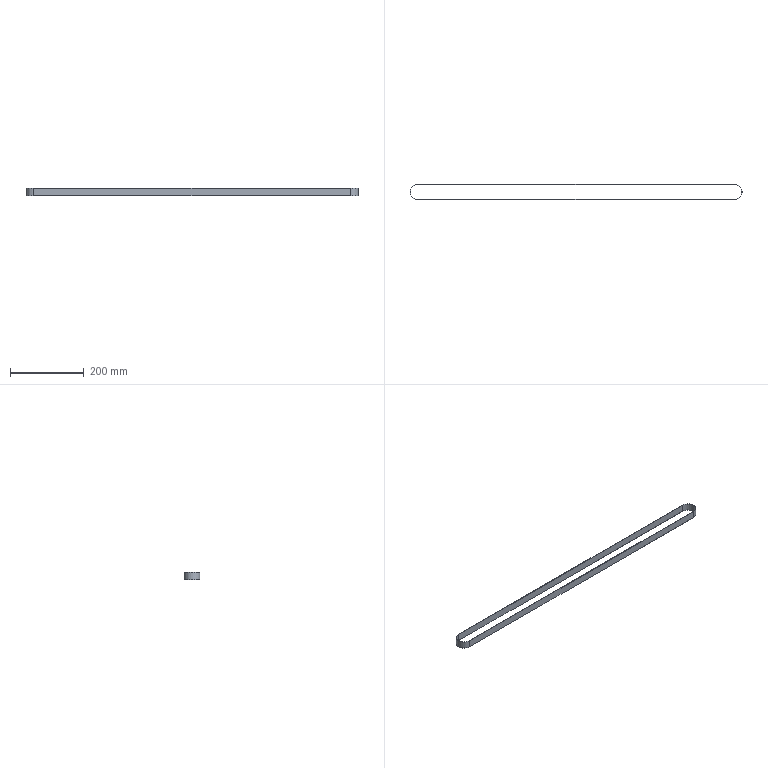Part | NX | 1 solid | 10 faces | box 898.6 x 42.6 x 20 mm | volume 36854 mm3 | plane 6 | cylinder 4 | commonest cylinder face diameters 40.6 x2 42.6 x2
STEP:
#1=CARTESIAN_POINT('',(-110.48,73.3,10.));
#2=VERTEX_POINT('',#1);
#3=CARTESIAN_POINT('',(-110.48,30.7,10.));
#4=VERTEX_POINT('',#3);
#5=CARTESIAN_POINT('',(-110.48,52.,10.));
#6=DIRECTION('',(0.,0.,-1.));
#7=DIRECTION('',(-1.,0.,0.));
#8=AXIS2_PLACEMENT_3D('',#5,#6,#7);
#9=CIRCLE('',#8,21.3);
#10=EDGE_CURVE('',#2,#4,#9,.F.);
#11=ORIENTED_EDGE('',*,*,#10,.T.);
#12=CARTESIAN_POINT('',(745.52,30.7,10.));
#13=VERTEX_POINT('',#12);
#14=CARTESIAN_POINT('',(-110.48,30.7,10.));
#15=DIRECTION('',(1.,0.,0.));
#16=VECTOR('',#15,1000.);
#17=LINE('',#14,#16);
#18=EDGE_CURVE('',#4,#13,#17,.T.);
#19=ORIENTED_EDGE('',*,*,#18,.T.);
#20=CARTESIAN_POINT('',(745.52,73.3,10.));
#21=VERTEX_POINT('',#20);
#22=CARTESIAN_POINT('',(745.52,52.,10.));
#23=DIRECTION('',(0.,0.,-1.));
#24=DIRECTION('',(-1.,0.,0.));
#25=AXIS2_PLACEMENT_3D('',#22,#23,#24);
#26=CIRCLE('',#25,21.3);
#27=EDGE_CURVE('',#13,#21,#26,.F.);
#28=ORIENTED_EDGE('',*,*,#27,.T.);
#29=CARTESIAN_POINT('',(-110.48,73.3,10.));
#30=DIRECTION('',(-1.,0.,0.));
#31=VECTOR('',#30,1000.);
#32=LINE('',#29,#31);
#33=EDGE_CURVE('',#21,#2,#32,.T.);
#34=ORIENTED_EDGE('',*,*,#33,.T.);
#35=EDGE_LOOP('',(#11,#19,#28,#34));
#36=FACE_BOUND('',#35,.T.);
#37=CARTESIAN_POINT('',(-110.48,72.3,10.));
#38=VERTEX_POINT('',#37);
#39=CARTESIAN_POINT('',(-110.48,31.7,10.));
#40=VERTEX_POINT('',#39);
#41=CARTESIAN_POINT('',(-110.48,52.,10.));
#42=DIRECTION('',(0.,0.,1.));
#43=DIRECTION('',(-1.,0.,0.));
#44=AXIS2_PLACEMENT_3D('',#41,#42,#43);
#45=CIRCLE('',#44,20.3);
#46=EDGE_CURVE('',#38,#40,#45,.T.);
#47=ORIENTED_EDGE('',*,*,#46,.F.);
#48=CARTESIAN_POINT('',(745.52,72.3,10.));
#49=VERTEX_POINT('',#48);
#50=CARTESIAN_POINT('',(-110.48,72.3,10.));
#51=DIRECTION('',(-1.,0.,0.));
#52=VECTOR('',#51,1000.);
#53=LINE('',#50,#52);
#54=EDGE_CURVE('',#49,#38,#53,.T.);
#55=ORIENTED_EDGE('',*,*,#54,.F.);
#56=CARTESIAN_POINT('',(745.52,31.7,10.));
#57=VERTEX_POINT('',#56);
#58=CARTESIAN_POINT('',(745.52,52.,10.));
#59=DIRECTION('',(0.,0.,1.));
#60=DIRECTION('',(-1.,0.,0.));
#61=AXIS2_PLACEMENT_3D('',#58,#59,#60);
#62=CIRCLE('',#61,20.3);
#63=EDGE_CURVE('',#57,#49,#62,.T.);
#64=ORIENTED_EDGE('',*,*,#63,.F.);
#65=CARTESIAN_POINT('',(745.52,31.7,10.));
#66=DIRECTION('',(1.,0.,0.));
#67=VECTOR('',#66,1000.);
#68=LINE('',#65,#67);
#69=EDGE_CURVE('',#40,#57,#68,.T.);
#70=ORIENTED_EDGE('',*,*,#69,.F.);
#71=EDGE_LOOP('',(#47,#55,#64,#70));
#72=FACE_BOUND('',#71,.T.);
#73=CARTESIAN_POINT('',(-110.48,52.,10.));
#74=DIRECTION('',(0.,0.,-1.));
#75=DIRECTION('',(-1.,0.,0.));
#76=AXIS2_PLACEMENT_3D('',#73,#74,#75);
#77=PLANE('',#76);
#78=ADVANCED_FACE('',(#36,#72),#77,.F.);
#79=CARTESIAN_POINT('',(-110.48,73.3,-10.));
#80=VERTEX_POINT('',#79);
#81=CARTESIAN_POINT('',(-110.48,30.7,-10.));
#82=VERTEX_POINT('',#81);
#83=CARTESIAN_POINT('',(-110.48,52.,-10.));
#84=DIRECTION('',(0.,0.,-1.));
#85=DIRECTION('',(-1.,0.,0.));
#86=AXIS2_PLACEMENT_3D('',#83,#84,#85);
#87=CIRCLE('',#86,21.3);
#88=EDGE_CURVE('',#80,#82,#87,.F.);
#89=ORIENTED_EDGE('',*,*,#88,.F.);
#90=CARTESIAN_POINT('',(745.52,73.3,-10.));
#91=VERTEX_POINT('',#90);
#92=CARTESIAN_POINT('',(-110.48,73.3,-10.));
#93=DIRECTION('',(-1.,0.,0.));
#94=VECTOR('',#93,1000.);
#95=LINE('',#92,#94);
#96=EDGE_CURVE('',#91,#80,#95,.T.);
#97=ORIENTED_EDGE('',*,*,#96,.F.);
#98=CARTESIAN_POINT('',(745.52,30.7,-10.));
#99=VERTEX_POINT('',#98);
#100=CARTESIAN_POINT('',(745.52,52.,-10.));
#101=DIRECTION('',(0.,0.,-1.));
#102=DIRECTION('',(-1.,0.,0.));
#103=AXIS2_PLACEMENT_3D('',#100,#101,#102);
#104=CIRCLE('',#103,21.3);
#105=EDGE_CURVE('',#99,#91,#104,.F.);
#106=ORIENTED_EDGE('',*,*,#105,.F.);
#107=CARTESIAN_POINT('',(-110.48,30.7,-10.));
#108=DIRECTION('',(1.,0.,0.));
#109=VECTOR('',#108,1000.);
#110=LINE('',#107,#109);
#111=EDGE_CURVE('',#82,#99,#110,.T.);
#112=ORIENTED_EDGE('',*,*,#111,.F.);
#113=EDGE_LOOP('',(#89,#97,#106,#112));
#114=FACE_BOUND('',#113,.T.);
#115=CARTESIAN_POINT('',(745.52,72.3,-10.));
#116=VERTEX_POINT('',#115);
#117=CARTESIAN_POINT('',(-110.48,72.3,-10.));
#118=VERTEX_POINT('',#117);
#119=CARTESIAN_POINT('',(-110.48,72.3,-10.));
#120=DIRECTION('',(-1.,0.,0.));
#121=VECTOR('',#120,1000.);
#122=LINE('',#119,#121);
#123=EDGE_CURVE('',#116,#118,#122,.T.);
#124=ORIENTED_EDGE('',*,*,#123,.T.);
#125=CARTESIAN_POINT('',(-110.48,31.7,-10.));
#126=VERTEX_POINT('',#125);
#127=CARTESIAN_POINT('',(-110.48,52.,-10.));
#128=DIRECTION('',(0.,0.,1.));
#129=DIRECTION('',(-1.,0.,0.));
#130=AXIS2_PLACEMENT_3D('',#127,#128,#129);
#131=CIRCLE('',#130,20.3);
#132=EDGE_CURVE('',#118,#126,#131,.T.);
#133=ORIENTED_EDGE('',*,*,#132,.T.);
#134=CARTESIAN_POINT('',(745.52,31.7,-10.));
#135=VERTEX_POINT('',#134);
#136=CARTESIAN_POINT('',(745.52,31.7,-10.));
#137=DIRECTION('',(1.,0.,0.));
#138=VECTOR('',#137,1000.);
#139=LINE('',#136,#138);
#140=EDGE_CURVE('',#126,#135,#139,.T.);
#141=ORIENTED_EDGE('',*,*,#140,.T.);
#142=CARTESIAN_POINT('',(745.52,52.,-10.));
#143=DIRECTION('',(0.,0.,1.));
#144=DIRECTION('',(-1.,0.,0.));
#145=AXIS2_PLACEMENT_3D('',#142,#143,#144);
#146=CIRCLE('',#145,20.3);
#147=EDGE_CURVE('',#135,#116,#146,.T.);
#148=ORIENTED_EDGE('',*,*,#147,.T.);
#149=EDGE_LOOP('',(#124,#133,#141,#148));
#150=FACE_BOUND('',#149,.T.);
#151=CARTESIAN_POINT('',(-110.48,52.,-10.));
#152=DIRECTION('',(0.,0.,-1.));
#153=DIRECTION('',(-1.,0.,0.));
#154=AXIS2_PLACEMENT_3D('',#151,#152,#153);
#155=PLANE('',#154);
#156=ADVANCED_FACE('',(#114,#150),#155,.T.);
#157=ORIENTED_EDGE('',*,*,#88,.T.);
#158=CARTESIAN_POINT('',(-110.48,30.7,10.));
#159=DIRECTION('',(0.,0.,-1.));
#160=VECTOR('',#159,1000.);
#161=LINE('',#158,#160);
#162=EDGE_CURVE('',#4,#82,#161,.T.);
#163=ORIENTED_EDGE('',*,*,#162,.F.);
#164=ORIENTED_EDGE('',*,*,#10,.F.);
#165=CARTESIAN_POINT('',(-110.48,73.3,10.));
#166=DIRECTION('',(0.,0.,-1.));
#167=VECTOR('',#166,1000.);
#168=LINE('',#165,#167);
#169=EDGE_CURVE('',#2,#80,#168,.T.);
#170=ORIENTED_EDGE('',*,*,#169,.T.);
#171=EDGE_LOOP('',(#157,#163,#164,#170));
#172=FACE_BOUND('',#171,.T.);
#173=CARTESIAN_POINT('',(-110.48,52.,10.));
#174=DIRECTION('',(0.,0.,-1.));
#175=DIRECTION('',(-1.,0.,0.));
#176=AXIS2_PLACEMENT_3D('',#173,#174,#175);
#177=CYLINDRICAL_SURFACE('',#176,21.3);
#178=ADVANCED_FACE('',(#172),#177,.T.);
#179=ORIENTED_EDGE('',*,*,#111,.T.);
#180=CARTESIAN_POINT('',(745.52,30.7,10.));
#181=DIRECTION('',(0.,0.,-1.));
#182=VECTOR('',#181,1000.);
#183=LINE('',#180,#182);
#184=EDGE_CURVE('',#13,#99,#183,.T.);
#185=ORIENTED_EDGE('',*,*,#184,.F.);
#186=ORIENTED_EDGE('',*,*,#18,.F.);
#187=ORIENTED_EDGE('',*,*,#162,.T.);
#188=EDGE_LOOP('',(#179,#185,#186,#187));
#189=FACE_BOUND('',#188,.T.);
#190=CARTESIAN_POINT('',(-110.48,30.7,10.));
#191=DIRECTION('',(0.,1.,0.));
#192=DIRECTION('',(-1.,0.,0.));
#193=AXIS2_PLACEMENT_3D('',#190,#191,#192);
#194=PLANE('',#193);
#195=ADVANCED_FACE('',(#189),#194,.F.);
#196=ORIENTED_EDGE('',*,*,#105,.T.);
#197=CARTESIAN_POINT('',(745.52,73.3,10.));
#198=DIRECTION('',(0.,0.,-1.));
#199=VECTOR('',#198,1000.);
#200=LINE('',#197,#199);
#201=EDGE_CURVE('',#21,#91,#200,.T.);
#202=ORIENTED_EDGE('',*,*,#201,.F.);
#203=ORIENTED_EDGE('',*,*,#27,.F.);
#204=ORIENTED_EDGE('',*,*,#184,.T.);
#205=EDGE_LOOP('',(#196,#202,#203,#204));
#206=FACE_BOUND('',#205,.T.);
#207=CARTESIAN_POINT('',(745.52,52.,10.));
#208=DIRECTION('',(0.,0.,-1.));
#209=DIRECTION('',(-1.,0.,0.));
#210=AXIS2_PLACEMENT_3D('',#207,#208,#209);
#211=CYLINDRICAL_SURFACE('',#210,21.3);
#212=ADVANCED_FACE('',(#206),#211,.T.);
#213=ORIENTED_EDGE('',*,*,#96,.T.);
#214=ORIENTED_EDGE('',*,*,#169,.F.);
#215=ORIENTED_EDGE('',*,*,#33,.F.);
#216=ORIENTED_EDGE('',*,*,#201,.T.);
#217=EDGE_LOOP('',(#213,#214,#215,#216));
#218=FACE_BOUND('',#217,.T.);
#219=CARTESIAN_POINT('',(-110.48,73.3,10.));
#220=DIRECTION('',(0.,-1.,0.));
#221=DIRECTION('',(0.,0.,-1.));
#222=AXIS2_PLACEMENT_3D('',#219,#220,#221);
#223=PLANE('',#222);
#224=ADVANCED_FACE('',(#218),#223,.F.);
#225=ORIENTED_EDGE('',*,*,#132,.F.);
#226=CARTESIAN_POINT('',(-110.48,72.3,10.));
#227=DIRECTION('',(0.,0.,-1.));
#228=VECTOR('',#227,1000.);
#229=LINE('',#226,#228);
#230=EDGE_CURVE('',#38,#118,#229,.T.);
#231=ORIENTED_EDGE('',*,*,#230,.F.);
#232=ORIENTED_EDGE('',*,*,#46,.T.);
#233=CARTESIAN_POINT('',(-110.48,31.7,10.));
#234=DIRECTION('',(0.,0.,-1.));
#235=VECTOR('',#234,1000.);
#236=LINE('',#233,#235);
#237=EDGE_CURVE('',#40,#126,#236,.T.);
#238=ORIENTED_EDGE('',*,*,#237,.T.);
#239=EDGE_LOOP('',(#225,#231,#232,#238));
#240=FACE_BOUND('',#239,.T.);
#241=CARTESIAN_POINT('',(-110.48,52.,10.));
#242=DIRECTION('',(0.,0.,-1.));
#243=DIRECTION('',(-1.,0.,0.));
#244=AXIS2_PLACEMENT_3D('',#241,#242,#243);
#245=CYLINDRICAL_SURFACE('',#244,20.3);
#246=ADVANCED_FACE('',(#240),#245,.F.);
#247=ORIENTED_EDGE('',*,*,#140,.F.);
#248=ORIENTED_EDGE('',*,*,#237,.F.);
#249=ORIENTED_EDGE('',*,*,#69,.T.);
#250=CARTESIAN_POINT('',(745.52,31.7,10.));
#251=DIRECTION('',(0.,0.,-1.));
#252=VECTOR('',#251,1000.);
#253=LINE('',#250,#252);
#254=EDGE_CURVE('',#57,#135,#253,.T.);
#255=ORIENTED_EDGE('',*,*,#254,.T.);
#256=EDGE_LOOP('',(#247,#248,#249,#255));
#257=FACE_BOUND('',#256,.T.);
#258=CARTESIAN_POINT('',(745.52,31.7,10.));
#259=DIRECTION('',(0.,1.,0.));
#260=DIRECTION('',(-1.,0.,0.));
#261=AXIS2_PLACEMENT_3D('',#258,#259,#260);
#262=PLANE('',#261);
#263=ADVANCED_FACE('',(#257),#262,.T.);
#264=ORIENTED_EDGE('',*,*,#147,.F.);
#265=ORIENTED_EDGE('',*,*,#254,.F.);
#266=ORIENTED_EDGE('',*,*,#63,.T.);
#267=CARTESIAN_POINT('',(745.52,72.3,10.));
#268=DIRECTION('',(0.,0.,-1.));
#269=VECTOR('',#268,1000.);
#270=LINE('',#267,#269);
#271=EDGE_CURVE('',#49,#116,#270,.T.);
#272=ORIENTED_EDGE('',*,*,#271,.T.);
#273=EDGE_LOOP('',(#264,#265,#266,#272));
#274=FACE_BOUND('',#273,.T.);
#275=CARTESIAN_POINT('',(745.52,52.,10.));
#276=DIRECTION('',(0.,0.,-1.));
#277=DIRECTION('',(-1.,0.,0.));
#278=AXIS2_PLACEMENT_3D('',#275,#276,#277);
#279=CYLINDRICAL_SURFACE('',#278,20.3);
#280=ADVANCED_FACE('',(#274),#279,.F.);
#281=ORIENTED_EDGE('',*,*,#123,.F.);
#282=ORIENTED_EDGE('',*,*,#271,.F.);
#283=ORIENTED_EDGE('',*,*,#54,.T.);
#284=ORIENTED_EDGE('',*,*,#230,.T.);
#285=EDGE_LOOP('',(#281,#282,#283,#284));
#286=FACE_BOUND('',#285,.T.);
#287=CARTESIAN_POINT('',(-110.48,72.3,10.));
#288=DIRECTION('',(0.,-1.,0.));
#289=DIRECTION('',(0.,0.,-1.));
#290=AXIS2_PLACEMENT_3D('',#287,#288,#289);
#291=PLANE('',#290);
#292=ADVANCED_FACE('',(#286),#291,.T.);
#293=CLOSED_SHELL('',(#78,#156,#178,#195,#212,#224,#246,#263,#280,#292));
#294=MANIFOLD_SOLID_BREP('',#293);
#295=(LENGTH_UNIT()NAMED_UNIT(*)SI_UNIT(.MILLI.,.METRE.));
#296=UNCERTAINTY_MEASURE_WITH_UNIT(LENGTH_MEASURE(0.00001),#295,'','');
#297=(NAMED_UNIT(*)PLANE_ANGLE_UNIT()SI_UNIT($,.RADIAN.));
#298=(NAMED_UNIT(*)SI_UNIT($,.STERADIAN.)SOLID_ANGLE_UNIT());
#299=(GEOMETRIC_REPRESENTATION_CONTEXT(3)GLOBAL_UNCERTAINTY_ASSIGNED_CONTEXT((#296))GLOBAL_UNIT_ASSIGNED_CONTEXT((#295,#297,#298))REPRESENTATION_CONTEXT('',''));
#300=ADVANCED_BREP_SHAPE_REPRESENTATION('',(#294),#299);